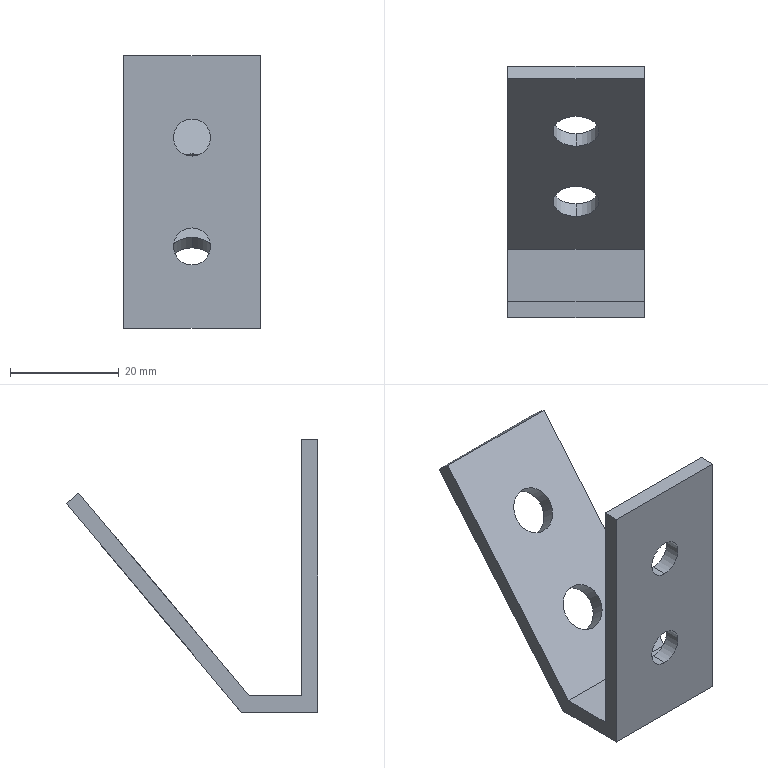Part | SolidWorks | features BaseBody 1 | 1 solid | 18 faces | box 25 x 46.139 x 50 mm | volume 7662 mm3 | plane 10 | cylinder 8 | commonest cylinder face diameters 6.8 x4 8.5 x4
STEP:
#1=CARTESIAN_POINT('',(0.,18.66,-416.173));
#2=VERTEX_POINT('',#1);
#3=CARTESIAN_POINT('',(0.,18.66,-422.973));
#4=VERTEX_POINT('',#3);
#5=CARTESIAN_POINT('',(0.,18.66,-419.573));
#6=DIRECTION('',(0.,-1.,0.));
#7=DIRECTION('',(0.,0.,-1.));
#8=AXIS2_PLACEMENT_3D('',#5,#6,#7);
#9=CIRCLE('',#8,3.4);
#10=EDGE_CURVE('',#2,#4,#9,.T.);
#11=ORIENTED_EDGE('',*,*,#10,.F.);
#12=CARTESIAN_POINT('',(0.,15.66,-416.173));
#13=VERTEX_POINT('',#12);
#14=CARTESIAN_POINT('',(0.,15.66,-416.173));
#15=DIRECTION('',(0.,-1.,0.));
#16=VECTOR('',#15,1000.);
#17=LINE('',#14,#16);
#18=EDGE_CURVE('',#2,#13,#17,.T.);
#19=ORIENTED_EDGE('',*,*,#18,.T.);
#20=CARTESIAN_POINT('',(0.,15.66,-422.973));
#21=VERTEX_POINT('',#20);
#22=CARTESIAN_POINT('',(0.,15.66,-419.573));
#23=DIRECTION('',(0.,-1.,0.));
#24=DIRECTION('',(0.,0.,-1.));
#25=AXIS2_PLACEMENT_3D('',#22,#23,#24);
#26=CIRCLE('',#25,3.4);
#27=EDGE_CURVE('',#13,#21,#26,.T.);
#28=ORIENTED_EDGE('',*,*,#27,.T.);
#29=CARTESIAN_POINT('',(0.,15.66,-422.973));
#30=DIRECTION('',(0.,-1.,0.));
#31=VECTOR('',#30,1000.);
#32=LINE('',#29,#31);
#33=EDGE_CURVE('',#4,#21,#32,.T.);
#34=ORIENTED_EDGE('',*,*,#33,.F.);
#35=EDGE_LOOP('',(#11,#19,#28,#34));
#36=FACE_OUTER_BOUND('',#35,.T.);
#37=CARTESIAN_POINT('',(0.,15.66,-419.573));
#38=DIRECTION('',(0.,-1.,0.));
#39=DIRECTION('',(0.,0.,-1.));
#40=AXIS2_PLACEMENT_3D('',#37,#38,#39);
#41=CYLINDRICAL_SURFACE('',#40,3.4);
#42=ADVANCED_FACE('',(#36),#41,.F.);
#43=CARTESIAN_POINT('',(0.,18.66,-396.173));
#44=VERTEX_POINT('',#43);
#45=CARTESIAN_POINT('',(0.,18.66,-402.973));
#46=VERTEX_POINT('',#45);
#47=CARTESIAN_POINT('',(0.,18.66,-399.573));
#48=DIRECTION('',(0.,-1.,0.));
#49=DIRECTION('',(0.,0.,-1.));
#50=AXIS2_PLACEMENT_3D('',#47,#48,#49);
#51=CIRCLE('',#50,3.4);
#52=EDGE_CURVE('',#44,#46,#51,.T.);
#53=ORIENTED_EDGE('',*,*,#52,.F.);
#54=CARTESIAN_POINT('',(0.,15.66,-396.173));
#55=VERTEX_POINT('',#54);
#56=CARTESIAN_POINT('',(0.,15.66,-396.173));
#57=DIRECTION('',(0.,-1.,0.));
#58=VECTOR('',#57,1000.);
#59=LINE('',#56,#58);
#60=EDGE_CURVE('',#44,#55,#59,.T.);
#61=ORIENTED_EDGE('',*,*,#60,.T.);
#62=CARTESIAN_POINT('',(0.,15.66,-402.973));
#63=VERTEX_POINT('',#62);
#64=CARTESIAN_POINT('',(0.,15.66,-399.573));
#65=DIRECTION('',(0.,-1.,0.));
#66=DIRECTION('',(0.,0.,-1.));
#67=AXIS2_PLACEMENT_3D('',#64,#65,#66);
#68=CIRCLE('',#67,3.4);
#69=EDGE_CURVE('',#55,#63,#68,.T.);
#70=ORIENTED_EDGE('',*,*,#69,.T.);
#71=CARTESIAN_POINT('',(0.,15.66,-402.973));
#72=DIRECTION('',(0.,-1.,0.));
#73=VECTOR('',#72,1000.);
#74=LINE('',#71,#73);
#75=EDGE_CURVE('',#46,#63,#74,.T.);
#76=ORIENTED_EDGE('',*,*,#75,.F.);
#77=EDGE_LOOP('',(#53,#61,#70,#76));
#78=FACE_OUTER_BOUND('',#77,.T.);
#79=CARTESIAN_POINT('',(0.,15.66,-399.573));
#80=DIRECTION('',(0.,-1.,0.));
#81=DIRECTION('',(0.,0.,-1.));
#82=AXIS2_PLACEMENT_3D('',#79,#80,#81);
#83=CYLINDRICAL_SURFACE('',#82,3.4);
#84=ADVANCED_FACE('',(#78),#83,.F.);
#85=CARTESIAN_POINT('',(0.,52.591,-402.577));
#86=VERTEX_POINT('',#85);
#87=CARTESIAN_POINT('',(0.,47.128,-409.089));
#88=VERTEX_POINT('',#87);
#89=CARTESIAN_POINT('',(0.,49.86,-405.833));
#90=DIRECTION('',(0.,-0.766,0.6428));
#91=DIRECTION('',(0.,0.6428,0.766));
#92=AXIS2_PLACEMENT_3D('',#89,#90,#91);
#93=CIRCLE('',#92,4.25);
#94=EDGE_CURVE('',#86,#88,#93,.T.);
#95=ORIENTED_EDGE('',*,*,#94,.T.);
#96=CARTESIAN_POINT('',(0.,49.426,-411.017));
#97=VERTEX_POINT('',#96);
#98=CARTESIAN_POINT('',(0.,46.362,-408.446));
#99=DIRECTION('',(0.,0.766,-0.6428));
#100=VECTOR('',#99,1000.);
#101=LINE('',#98,#100);
#102=EDGE_CURVE('',#88,#97,#101,.T.);
#103=ORIENTED_EDGE('',*,*,#102,.T.);
#104=CARTESIAN_POINT('',(0.,54.89,-404.506));
#105=VERTEX_POINT('',#104);
#106=CARTESIAN_POINT('',(0.,52.158,-407.761));
#107=DIRECTION('',(0.,0.766,-0.6428));
#108=DIRECTION('',(0.,0.6428,0.766));
#109=AXIS2_PLACEMENT_3D('',#106,#107,#108);
#110=CIRCLE('',#109,4.25);
#111=EDGE_CURVE('',#97,#105,#110,.T.);
#112=ORIENTED_EDGE('',*,*,#111,.T.);
#113=CARTESIAN_POINT('',(0.,51.825,-401.934));
#114=DIRECTION('',(0.,0.766,-0.6428));
#115=VECTOR('',#114,1000.);
#116=LINE('',#113,#115);
#117=EDGE_CURVE('',#86,#105,#116,.T.);
#118=ORIENTED_EDGE('',*,*,#117,.F.);
#119=EDGE_LOOP('',(#95,#103,#112,#118));
#120=FACE_OUTER_BOUND('',#119,.T.);
#121=CARTESIAN_POINT('',(0.,49.093,-405.19));
#122=DIRECTION('',(0.,0.766,-0.6428));
#123=DIRECTION('',(0.,0.6428,0.766));
#124=AXIS2_PLACEMENT_3D('',#121,#122,#123);
#125=CYLINDRICAL_SURFACE('',#124,4.25);
#126=ADVANCED_FACE('',(#120),#125,.F.);
#127=CARTESIAN_POINT('',(0.,39.736,-417.898));
#128=VERTEX_POINT('',#127);
#129=CARTESIAN_POINT('',(0.,34.272,-424.409));
#130=VERTEX_POINT('',#129);
#131=CARTESIAN_POINT('',(0.,37.004,-421.154));
#132=DIRECTION('',(0.,-0.766,0.6428));
#133=DIRECTION('',(0.,0.6428,0.766));
#134=AXIS2_PLACEMENT_3D('',#131,#132,#133);
#135=CIRCLE('',#134,4.25);
#136=EDGE_CURVE('',#128,#130,#135,.T.);
#137=ORIENTED_EDGE('',*,*,#136,.T.);
#138=CARTESIAN_POINT('',(0.,36.57,-426.338));
#139=VERTEX_POINT('',#138);
#140=CARTESIAN_POINT('',(0.,33.506,-423.767));
#141=DIRECTION('',(0.,0.766,-0.6428));
#142=VECTOR('',#141,1000.);
#143=LINE('',#140,#142);
#144=EDGE_CURVE('',#130,#139,#143,.T.);
#145=ORIENTED_EDGE('',*,*,#144,.T.);
#146=CARTESIAN_POINT('',(0.,42.034,-419.826));
#147=VERTEX_POINT('',#146);
#148=CARTESIAN_POINT('',(0.,39.302,-423.082));
#149=DIRECTION('',(0.,0.766,-0.6428));
#150=DIRECTION('',(0.,0.6428,0.766));
#151=AXIS2_PLACEMENT_3D('',#148,#149,#150);
#152=CIRCLE('',#151,4.25);
#153=EDGE_CURVE('',#139,#147,#152,.T.);
#154=ORIENTED_EDGE('',*,*,#153,.T.);
#155=CARTESIAN_POINT('',(0.,38.97,-417.255));
#156=DIRECTION('',(0.,0.766,-0.6428));
#157=VECTOR('',#156,1000.);
#158=LINE('',#155,#157);
#159=EDGE_CURVE('',#128,#147,#158,.T.);
#160=ORIENTED_EDGE('',*,*,#159,.F.);
#161=EDGE_LOOP('',(#137,#145,#154,#160));
#162=FACE_OUTER_BOUND('',#161,.T.);
#163=CARTESIAN_POINT('',(0.,36.238,-420.511));
#164=DIRECTION('',(0.,0.766,-0.6428));
#165=DIRECTION('',(0.,0.6428,0.766));
#166=AXIS2_PLACEMENT_3D('',#163,#164,#165);
#167=CYLINDRICAL_SURFACE('',#166,4.25);
#168=ADVANCED_FACE('',(#162),#167,.F.);
#169=CARTESIAN_POINT('',(0.,15.66,-419.573));
#170=DIRECTION('',(0.,-1.,0.));
#171=DIRECTION('',(0.,0.,-1.));
#172=AXIS2_PLACEMENT_3D('',#169,#170,#171);
#173=CIRCLE('',#172,3.4);
#174=EDGE_CURVE('',#21,#13,#173,.T.);
#175=ORIENTED_EDGE('',*,*,#174,.F.);
#176=ORIENTED_EDGE('',*,*,#27,.F.);
#177=EDGE_LOOP('',(#175,#176));
#178=FACE_BOUND('',#177,.T.);
#179=CARTESIAN_POINT('',(12.5,15.66,-434.573));
#180=VERTEX_POINT('',#179);
#181=CARTESIAN_POINT('',(-12.5,15.66,-434.573));
#182=VERTEX_POINT('',#181);
#183=CARTESIAN_POINT('',(12.5,15.66,-434.573));
#184=DIRECTION('',(-1.,0.,0.));
#185=VECTOR('',#184,1000.);
#186=LINE('',#183,#185);
#187=EDGE_CURVE('',#180,#182,#186,.T.);
#188=ORIENTED_EDGE('',*,*,#187,.F.);
#189=CARTESIAN_POINT('',(12.5,15.66,-384.573));
#190=VERTEX_POINT('',#189);
#191=CARTESIAN_POINT('',(12.5,15.66,-434.573));
#192=DIRECTION('',(0.,0.,-1.));
#193=VECTOR('',#192,1000.);
#194=LINE('',#191,#193);
#195=EDGE_CURVE('',#190,#180,#194,.T.);
#196=ORIENTED_EDGE('',*,*,#195,.F.);
#197=CARTESIAN_POINT('',(-12.5,15.66,-384.573));
#198=VERTEX_POINT('',#197);
#199=CARTESIAN_POINT('',(12.5,15.66,-384.573));
#200=DIRECTION('',(1.,0.,0.));
#201=VECTOR('',#200,1000.);
#202=LINE('',#199,#201);
#203=EDGE_CURVE('',#198,#190,#202,.T.);
#204=ORIENTED_EDGE('',*,*,#203,.F.);
#205=CARTESIAN_POINT('',(-12.5,15.66,-434.573));
#206=DIRECTION('',(0.,0.,1.));
#207=VECTOR('',#206,1000.);
#208=LINE('',#205,#207);
#209=EDGE_CURVE('',#182,#198,#208,.T.);
#210=ORIENTED_EDGE('',*,*,#209,.F.);
#211=EDGE_LOOP('',(#188,#196,#204,#210));
#212=FACE_OUTER_BOUND('',#211,.T.);
#213=CARTESIAN_POINT('',(0.,15.66,-399.573));
#214=DIRECTION('',(0.,-1.,0.));
#215=DIRECTION('',(0.,0.,-1.));
#216=AXIS2_PLACEMENT_3D('',#213,#214,#215);
#217=CIRCLE('',#216,3.4);
#218=EDGE_CURVE('',#63,#55,#217,.T.);
#219=ORIENTED_EDGE('',*,*,#218,.F.);
#220=ORIENTED_EDGE('',*,*,#69,.F.);
#221=EDGE_LOOP('',(#219,#220));
#222=FACE_BOUND('',#221,.T.);
#223=CARTESIAN_POINT('',(12.5,15.66,-434.573));
#224=DIRECTION('',(0.,1.,0.));
#225=DIRECTION('',(0.,0.,1.));
#226=AXIS2_PLACEMENT_3D('',#223,#224,#225);
#227=PLANE('',#226);
#228=ADVANCED_FACE('',(#178,#212,#222),#227,.F.);
#229=ORIENTED_EDGE('',*,*,#18,.F.);
#230=CARTESIAN_POINT('',(0.,18.66,-419.573));
#231=DIRECTION('',(0.,-1.,0.));
#232=DIRECTION('',(0.,0.,-1.));
#233=AXIS2_PLACEMENT_3D('',#230,#231,#232);
#234=CIRCLE('',#233,3.4);
#235=EDGE_CURVE('',#4,#2,#234,.T.);
#236=ORIENTED_EDGE('',*,*,#235,.F.);
#237=ORIENTED_EDGE('',*,*,#33,.T.);
#238=ORIENTED_EDGE('',*,*,#174,.T.);
#239=EDGE_LOOP('',(#229,#236,#237,#238));
#240=FACE_OUTER_BOUND('',#239,.T.);
#241=CARTESIAN_POINT('',(0.,15.66,-419.573));
#242=DIRECTION('',(0.,-1.,0.));
#243=DIRECTION('',(0.,0.,-1.));
#244=AXIS2_PLACEMENT_3D('',#241,#242,#243);
#245=CYLINDRICAL_SURFACE('',#244,3.4);
#246=ADVANCED_FACE('',(#240),#245,.F.);
#247=CARTESIAN_POINT('',(-12.5,29.66,-434.573));
#248=VERTEX_POINT('',#247);
#249=CARTESIAN_POINT('',(-12.5,61.799,-396.271));
#250=VERTEX_POINT('',#249);
#251=CARTESIAN_POINT('',(-12.5,29.66,-434.573));
#252=DIRECTION('',(0.,0.6428,0.766));
#253=VECTOR('',#252,1000.);
#254=LINE('',#251,#253);
#255=EDGE_CURVE('',#248,#250,#254,.T.);
#256=ORIENTED_EDGE('',*,*,#255,.F.);
#257=CARTESIAN_POINT('',(-12.5,10.117,-434.573));
#258=DIRECTION('',(0.,1.,0.));
#259=VECTOR('',#258,1000.);
#260=LINE('',#257,#259);
#261=EDGE_CURVE('',#182,#248,#260,.T.);
#262=ORIENTED_EDGE('',*,*,#261,.F.);
#263=ORIENTED_EDGE('',*,*,#209,.T.);
#264=CARTESIAN_POINT('',(-12.5,18.66,-384.573));
#265=VERTEX_POINT('',#264);
#266=CARTESIAN_POINT('',(-12.5,10.117,-384.573));
#267=DIRECTION('',(0.,-1.,0.));
#268=VECTOR('',#267,1000.);
#269=LINE('',#266,#268);
#270=EDGE_CURVE('',#265,#198,#269,.T.);
#271=ORIENTED_EDGE('',*,*,#270,.F.);
#272=CARTESIAN_POINT('',(-12.5,18.66,-431.573));
#273=VERTEX_POINT('',#272);
#274=CARTESIAN_POINT('',(-12.5,18.66,-407.196));
#275=DIRECTION('',(0.,0.,1.));
#276=VECTOR('',#275,1000.);
#277=LINE('',#274,#276);
#278=EDGE_CURVE('',#273,#265,#277,.T.);
#279=ORIENTED_EDGE('',*,*,#278,.F.);
#280=CARTESIAN_POINT('',(-12.5,28.261,-431.573));
#281=VERTEX_POINT('',#280);
#282=CARTESIAN_POINT('',(-12.5,10.117,-431.573));
#283=DIRECTION('',(0.,-1.,0.));
#284=VECTOR('',#283,1000.);
#285=LINE('',#282,#284);
#286=EDGE_CURVE('',#281,#273,#285,.T.);
#287=ORIENTED_EDGE('',*,*,#286,.F.);
#288=CARTESIAN_POINT('',(-12.5,59.501,-394.342));
#289=VERTEX_POINT('',#288);
#290=CARTESIAN_POINT('',(-12.5,59.501,-394.342));
#291=DIRECTION('',(0.,-0.6428,-0.766));
#292=VECTOR('',#291,1000.);
#293=LINE('',#290,#292);
#294=EDGE_CURVE('',#289,#281,#293,.T.);
#295=ORIENTED_EDGE('',*,*,#294,.F.);
#296=CARTESIAN_POINT('',(-12.5,61.799,-396.271));
#297=DIRECTION('',(0.,-0.766,0.6428));
#298=VECTOR('',#297,1000.);
#299=LINE('',#296,#298);
#300=EDGE_CURVE('',#250,#289,#299,.T.);
#301=ORIENTED_EDGE('',*,*,#300,.F.);
#302=EDGE_LOOP('',(#256,#262,#263,#271,#279,#287,#295,#301));
#303=FACE_OUTER_BOUND('',#302,.T.);
#304=CARTESIAN_POINT('',(-12.5,10.117,-407.196));
#305=DIRECTION('',(1.,0.,0.));
#306=DIRECTION('',(0.,0.,-1.));
#307=AXIS2_PLACEMENT_3D('',#304,#305,#306);
#308=PLANE('',#307);
#309=ADVANCED_FACE('',(#303),#308,.F.);
#310=CARTESIAN_POINT('',(12.5,29.66,-434.573));
#311=VERTEX_POINT('',#310);
#312=CARTESIAN_POINT('',(12.5,29.66,-434.573));
#313=DIRECTION('',(-1.,0.,0.));
#314=VECTOR('',#313,1000.);
#315=LINE('',#312,#314);
#316=EDGE_CURVE('',#311,#248,#315,.T.);
#317=ORIENTED_EDGE('',*,*,#316,.F.);
#318=CARTESIAN_POINT('',(12.5,29.66,-434.573));
#319=DIRECTION('',(0.,1.,0.));
#320=VECTOR('',#319,1000.);
#321=LINE('',#318,#320);
#322=EDGE_CURVE('',#180,#311,#321,.T.);
#323=ORIENTED_EDGE('',*,*,#322,.F.);
#324=ORIENTED_EDGE('',*,*,#187,.T.);
#325=ORIENTED_EDGE('',*,*,#261,.T.);
#326=EDGE_LOOP('',(#317,#323,#324,#325));
#327=FACE_OUTER_BOUND('',#326,.T.);
#328=CARTESIAN_POINT('',(12.5,29.66,-434.573));
#329=DIRECTION('',(0.,0.,1.));
#330=DIRECTION('',(1.,0.,0.));
#331=AXIS2_PLACEMENT_3D('',#328,#329,#330);
#332=PLANE('',#331);
#333=ADVANCED_FACE('',(#327),#332,.F.);
#334=ORIENTED_EDGE('',*,*,#322,.T.);
#335=CARTESIAN_POINT('',(12.5,61.799,-396.271));
#336=VERTEX_POINT('',#335);
#337=CARTESIAN_POINT('',(12.5,29.66,-434.573));
#338=DIRECTION('',(0.,0.6428,0.766));
#339=VECTOR('',#338,1000.);
#340=LINE('',#337,#339);
#341=EDGE_CURVE('',#311,#336,#340,.T.);
#342=ORIENTED_EDGE('',*,*,#341,.T.);
#343=CARTESIAN_POINT('',(12.5,59.501,-394.342));
#344=VERTEX_POINT('',#343);
#345=CARTESIAN_POINT('',(12.5,61.799,-396.271));
#346=DIRECTION('',(0.,-0.766,0.6428));
#347=VECTOR('',#346,1000.);
#348=LINE('',#345,#347);
#349=EDGE_CURVE('',#336,#344,#348,.T.);
#350=ORIENTED_EDGE('',*,*,#349,.T.);
#351=CARTESIAN_POINT('',(12.5,28.261,-431.573));
#352=VERTEX_POINT('',#351);
#353=CARTESIAN_POINT('',(12.5,59.501,-394.342));
#354=DIRECTION('',(0.,-0.6428,-0.766));
#355=VECTOR('',#354,1000.);
#356=LINE('',#353,#355);
#357=EDGE_CURVE('',#344,#352,#356,.T.);
#358=ORIENTED_EDGE('',*,*,#357,.T.);
#359=CARTESIAN_POINT('',(12.5,18.66,-431.573));
#360=VERTEX_POINT('',#359);
#361=CARTESIAN_POINT('',(12.5,10.117,-431.573));
#362=DIRECTION('',(0.,-1.,0.));
#363=VECTOR('',#362,1000.);
#364=LINE('',#361,#363);
#365=EDGE_CURVE('',#352,#360,#364,.T.);
#366=ORIENTED_EDGE('',*,*,#365,.T.);
#367=CARTESIAN_POINT('',(12.5,18.66,-384.573));
#368=VERTEX_POINT('',#367);
#369=CARTESIAN_POINT('',(12.5,18.66,-407.196));
#370=DIRECTION('',(0.,0.,1.));
#371=VECTOR('',#370,1000.);
#372=LINE('',#369,#371);
#373=EDGE_CURVE('',#360,#368,#372,.T.);
#374=ORIENTED_EDGE('',*,*,#373,.T.);
#375=CARTESIAN_POINT('',(12.5,10.117,-384.573));
#376=DIRECTION('',(0.,-1.,0.));
#377=VECTOR('',#376,1000.);
#378=LINE('',#375,#377);
#379=EDGE_CURVE('',#368,#190,#378,.T.);
#380=ORIENTED_EDGE('',*,*,#379,.T.);
#381=ORIENTED_EDGE('',*,*,#195,.T.);
#382=EDGE_LOOP('',(#334,#342,#350,#358,#366,#374,#380,#381));
#383=FACE_OUTER_BOUND('',#382,.T.);
#384=CARTESIAN_POINT('',(12.5,10.117,-407.196));
#385=DIRECTION('',(1.,0.,0.));
#386=DIRECTION('',(0.,0.,-1.));
#387=AXIS2_PLACEMENT_3D('',#384,#385,#386);
#388=PLANE('',#387);
#389=ADVANCED_FACE('',(#383),#388,.T.);
#390=ORIENTED_EDGE('',*,*,#203,.T.);
#391=ORIENTED_EDGE('',*,*,#379,.F.);
#392=CARTESIAN_POINT('',(12.5,18.66,-384.573));
#393=DIRECTION('',(1.,0.,0.));
#394=VECTOR('',#393,1000.);
#395=LINE('',#392,#394);
#396=EDGE_CURVE('',#265,#368,#395,.T.);
#397=ORIENTED_EDGE('',*,*,#396,.F.);
#398=ORIENTED_EDGE('',*,*,#270,.T.);
#399=EDGE_LOOP('',(#390,#391,#397,#398));
#400=FACE_OUTER_BOUND('',#399,.T.);
#401=CARTESIAN_POINT('',(12.5,18.66,-384.573));
#402=DIRECTION('',(0.,0.,-1.));
#403=DIRECTION('',(-1.,0.,0.));
#404=AXIS2_PLACEMENT_3D('',#401,#402,#403);
#405=PLANE('',#404);
#406=ADVANCED_FACE('',(#400),#405,.F.);
#407=ORIENTED_EDGE('',*,*,#60,.F.);
#408=CARTESIAN_POINT('',(0.,18.66,-399.573));
#409=DIRECTION('',(0.,-1.,0.));
#410=DIRECTION('',(0.,0.,-1.));
#411=AXIS2_PLACEMENT_3D('',#408,#409,#410);
#412=CIRCLE('',#411,3.4);
#413=EDGE_CURVE('',#46,#44,#412,.T.);
#414=ORIENTED_EDGE('',*,*,#413,.F.);
#415=ORIENTED_EDGE('',*,*,#75,.T.);
#416=ORIENTED_EDGE('',*,*,#218,.T.);
#417=EDGE_LOOP('',(#407,#414,#415,#416));
#418=FACE_OUTER_BOUND('',#417,.T.);
#419=CARTESIAN_POINT('',(0.,15.66,-399.573));
#420=DIRECTION('',(0.,-1.,0.));
#421=DIRECTION('',(0.,0.,-1.));
#422=AXIS2_PLACEMENT_3D('',#419,#420,#421);
#423=CYLINDRICAL_SURFACE('',#422,3.4);
#424=ADVANCED_FACE('',(#418),#423,.F.);
#425=ORIENTED_EDGE('',*,*,#396,.T.);
#426=ORIENTED_EDGE('',*,*,#373,.F.);
#427=CARTESIAN_POINT('',(12.5,18.66,-431.573));
#428=DIRECTION('',(1.,0.,0.));
#429=VECTOR('',#428,1000.);
#430=LINE('',#427,#429);
#431=EDGE_CURVE('',#273,#360,#430,.T.);
#432=ORIENTED_EDGE('',*,*,#431,.F.);
#433=ORIENTED_EDGE('',*,*,#278,.T.);
#434=EDGE_LOOP('',(#425,#426,#432,#433));
#435=FACE_OUTER_BOUND('',#434,.T.);
#436=ORIENTED_EDGE('',*,*,#235,.T.);
#437=ORIENTED_EDGE('',*,*,#10,.T.);
#438=EDGE_LOOP('',(#436,#437));
#439=FACE_BOUND('',#438,.T.);
#440=ORIENTED_EDGE('',*,*,#413,.T.);
#441=ORIENTED_EDGE('',*,*,#52,.T.);
#442=EDGE_LOOP('',(#440,#441));
#443=FACE_BOUND('',#442,.T.);
#444=CARTESIAN_POINT('',(12.5,18.66,-431.573));
#445=DIRECTION('',(0.,-1.,0.));
#446=DIRECTION('',(0.,0.,-1.));
#447=AXIS2_PLACEMENT_3D('',#444,#445,#446);
#448=PLANE('',#447);
#449=ADVANCED_FACE('',(#435,#439,#443),#448,.F.);
#450=CARTESIAN_POINT('',(12.5,59.501,-394.342));
#451=DIRECTION('',(-1.,0.,0.));
#452=VECTOR('',#451,1000.);
#453=LINE('',#450,#452);
#454=EDGE_CURVE('',#344,#289,#453,.T.);
#455=ORIENTED_EDGE('',*,*,#454,.F.);
#456=ORIENTED_EDGE('',*,*,#349,.F.);
#457=CARTESIAN_POINT('',(12.5,61.799,-396.271));
#458=DIRECTION('',(1.,0.,0.));
#459=VECTOR('',#458,1000.);
#460=LINE('',#457,#459);
#461=EDGE_CURVE('',#250,#336,#460,.T.);
#462=ORIENTED_EDGE('',*,*,#461,.F.);
#463=ORIENTED_EDGE('',*,*,#300,.T.);
#464=EDGE_LOOP('',(#455,#456,#462,#463));
#465=FACE_OUTER_BOUND('',#464,.T.);
#466=CARTESIAN_POINT('',(12.5,61.799,-396.271));
#467=DIRECTION('',(0.,-0.6428,-0.766));
#468=DIRECTION('',(0.,0.766,-0.6428));
#469=AXIS2_PLACEMENT_3D('',#466,#467,#468);
#470=PLANE('',#469);
#471=ADVANCED_FACE('',(#465),#470,.F.);
#472=ORIENTED_EDGE('',*,*,#461,.T.);
#473=ORIENTED_EDGE('',*,*,#341,.F.);
#474=ORIENTED_EDGE('',*,*,#316,.T.);
#475=ORIENTED_EDGE('',*,*,#255,.T.);
#476=EDGE_LOOP('',(#472,#473,#474,#475));
#477=FACE_OUTER_BOUND('',#476,.T.);
#478=CARTESIAN_POINT('',(0.,52.158,-407.761));
#479=DIRECTION('',(0.,0.766,-0.6428));
#480=DIRECTION('',(0.,0.6428,0.766));
#481=AXIS2_PLACEMENT_3D('',#478,#479,#480);
#482=CIRCLE('',#481,4.25);
#483=EDGE_CURVE('',#105,#97,#482,.T.);
#484=ORIENTED_EDGE('',*,*,#483,.F.);
#485=ORIENTED_EDGE('',*,*,#111,.F.);
#486=EDGE_LOOP('',(#484,#485));
#487=FACE_BOUND('',#486,.T.);
#488=CARTESIAN_POINT('',(0.,39.302,-423.082));
#489=DIRECTION('',(0.,0.766,-0.6428));
#490=DIRECTION('',(0.,0.6428,0.766));
#491=AXIS2_PLACEMENT_3D('',#488,#489,#490);
#492=CIRCLE('',#491,4.25);
#493=EDGE_CURVE('',#147,#139,#492,.T.);
#494=ORIENTED_EDGE('',*,*,#493,.F.);
#495=ORIENTED_EDGE('',*,*,#153,.F.);
#496=EDGE_LOOP('',(#494,#495));
#497=FACE_BOUND('',#496,.T.);
#498=CARTESIAN_POINT('',(12.5,61.799,-396.271));
#499=DIRECTION('',(0.,-0.766,0.6428));
#500=DIRECTION('',(0.,-0.6428,-0.766));
#501=AXIS2_PLACEMENT_3D('',#498,#499,#500);
#502=PLANE('',#501);
#503=ADVANCED_FACE('',(#477,#487,#497),#502,.F.);
#504=ORIENTED_EDGE('',*,*,#431,.T.);
#505=ORIENTED_EDGE('',*,*,#365,.F.);
#506=CARTESIAN_POINT('',(12.5,28.261,-431.573));
#507=DIRECTION('',(1.,0.,0.));
#508=VECTOR('',#507,1000.);
#509=LINE('',#506,#508);
#510=EDGE_CURVE('',#281,#352,#509,.T.);
#511=ORIENTED_EDGE('',*,*,#510,.F.);
#512=ORIENTED_EDGE('',*,*,#286,.T.);
#513=EDGE_LOOP('',(#504,#505,#511,#512));
#514=FACE_OUTER_BOUND('',#513,.T.);
#515=CARTESIAN_POINT('',(12.5,28.261,-431.573));
#516=DIRECTION('',(0.,0.,-1.));
#517=DIRECTION('',(-1.,0.,0.));
#518=AXIS2_PLACEMENT_3D('',#515,#516,#517);
#519=PLANE('',#518);
#520=ADVANCED_FACE('',(#514),#519,.F.);
#521=ORIENTED_EDGE('',*,*,#510,.T.);
#522=ORIENTED_EDGE('',*,*,#357,.F.);
#523=ORIENTED_EDGE('',*,*,#454,.T.);
#524=ORIENTED_EDGE('',*,*,#294,.T.);
#525=EDGE_LOOP('',(#521,#522,#523,#524));
#526=FACE_OUTER_BOUND('',#525,.T.);
#527=ORIENTED_EDGE('',*,*,#94,.F.);
#528=CARTESIAN_POINT('',(0.,49.86,-405.833));
#529=DIRECTION('',(0.,-0.766,0.6428));
#530=DIRECTION('',(0.,0.6428,0.766));
#531=AXIS2_PLACEMENT_3D('',#528,#529,#530);
#532=CIRCLE('',#531,4.25);
#533=EDGE_CURVE('',#88,#86,#532,.T.);
#534=ORIENTED_EDGE('',*,*,#533,.F.);
#535=EDGE_LOOP('',(#527,#534));
#536=FACE_BOUND('',#535,.T.);
#537=ORIENTED_EDGE('',*,*,#136,.F.);
#538=CARTESIAN_POINT('',(0.,37.004,-421.154));
#539=DIRECTION('',(0.,-0.766,0.6428));
#540=DIRECTION('',(0.,0.6428,0.766));
#541=AXIS2_PLACEMENT_3D('',#538,#539,#540);
#542=CIRCLE('',#541,4.25);
#543=EDGE_CURVE('',#130,#128,#542,.T.);
#544=ORIENTED_EDGE('',*,*,#543,.F.);
#545=EDGE_LOOP('',(#537,#544));
#546=FACE_BOUND('',#545,.T.);
#547=CARTESIAN_POINT('',(12.5,59.501,-394.342));
#548=DIRECTION('',(0.,0.766,-0.6428));
#549=DIRECTION('',(0.,0.6428,0.766));
#550=AXIS2_PLACEMENT_3D('',#547,#548,#549);
#551=PLANE('',#550);
#552=ADVANCED_FACE('',(#526,#536,#546),#551,.F.);
#553=ORIENTED_EDGE('',*,*,#102,.F.);
#554=ORIENTED_EDGE('',*,*,#533,.T.);
#555=ORIENTED_EDGE('',*,*,#117,.T.);
#556=ORIENTED_EDGE('',*,*,#483,.T.);
#557=EDGE_LOOP('',(#553,#554,#555,#556));
#558=FACE_OUTER_BOUND('',#557,.T.);
#559=CARTESIAN_POINT('',(0.,49.093,-405.19));
#560=DIRECTION('',(0.,0.766,-0.6428));
#561=DIRECTION('',(0.,0.6428,0.766));
#562=AXIS2_PLACEMENT_3D('',#559,#560,#561);
#563=CYLINDRICAL_SURFACE('',#562,4.25);
#564=ADVANCED_FACE('',(#558),#563,.F.);
#565=ORIENTED_EDGE('',*,*,#144,.F.);
#566=ORIENTED_EDGE('',*,*,#543,.T.);
#567=ORIENTED_EDGE('',*,*,#159,.T.);
#568=ORIENTED_EDGE('',*,*,#493,.T.);
#569=EDGE_LOOP('',(#565,#566,#567,#568));
#570=FACE_OUTER_BOUND('',#569,.T.);
#571=CARTESIAN_POINT('',(0.,36.238,-420.511));
#572=DIRECTION('',(0.,0.766,-0.6428));
#573=DIRECTION('',(0.,0.6428,0.766));
#574=AXIS2_PLACEMENT_3D('',#571,#572,#573);
#575=CYLINDRICAL_SURFACE('',#574,4.25);
#576=ADVANCED_FACE('',(#570),#575,.F.);
#577=CLOSED_SHELL('',(#42,#84,#126,#168,#228,#246,#309,#333,#389,#406,#424,#449,#471,#503,#520,#552,#564,#576));
#578=MANIFOLD_SOLID_BREP('',#577);
#579=CARTESIAN_POINT('',(0.,0.,0.));
#580=DIRECTION('',(0.,0.,1.));
#581=DIRECTION('',(1.,0.,0.));
#582=AXIS2_PLACEMENT_3D('',#579,#580,#581);
#583=(LENGTH_UNIT()NAMED_UNIT(*)SI_UNIT(.MILLI.,.METRE.));
#584=UNCERTAINTY_MEASURE_WITH_UNIT(LENGTH_MEASURE(0.00001),#583,'','');
#585=(NAMED_UNIT(*)PLANE_ANGLE_UNIT()SI_UNIT($,.RADIAN.));
#586=(NAMED_UNIT(*)SI_UNIT($,.STERADIAN.)SOLID_ANGLE_UNIT());
#587=(GEOMETRIC_REPRESENTATION_CONTEXT(3)GLOBAL_UNCERTAINTY_ASSIGNED_CONTEXT((#584))GLOBAL_UNIT_ASSIGNED_CONTEXT((#583,#585,#586))REPRESENTATION_CONTEXT('',''));
#588=ADVANCED_BREP_SHAPE_REPRESENTATION('',(#578,#582),#587);